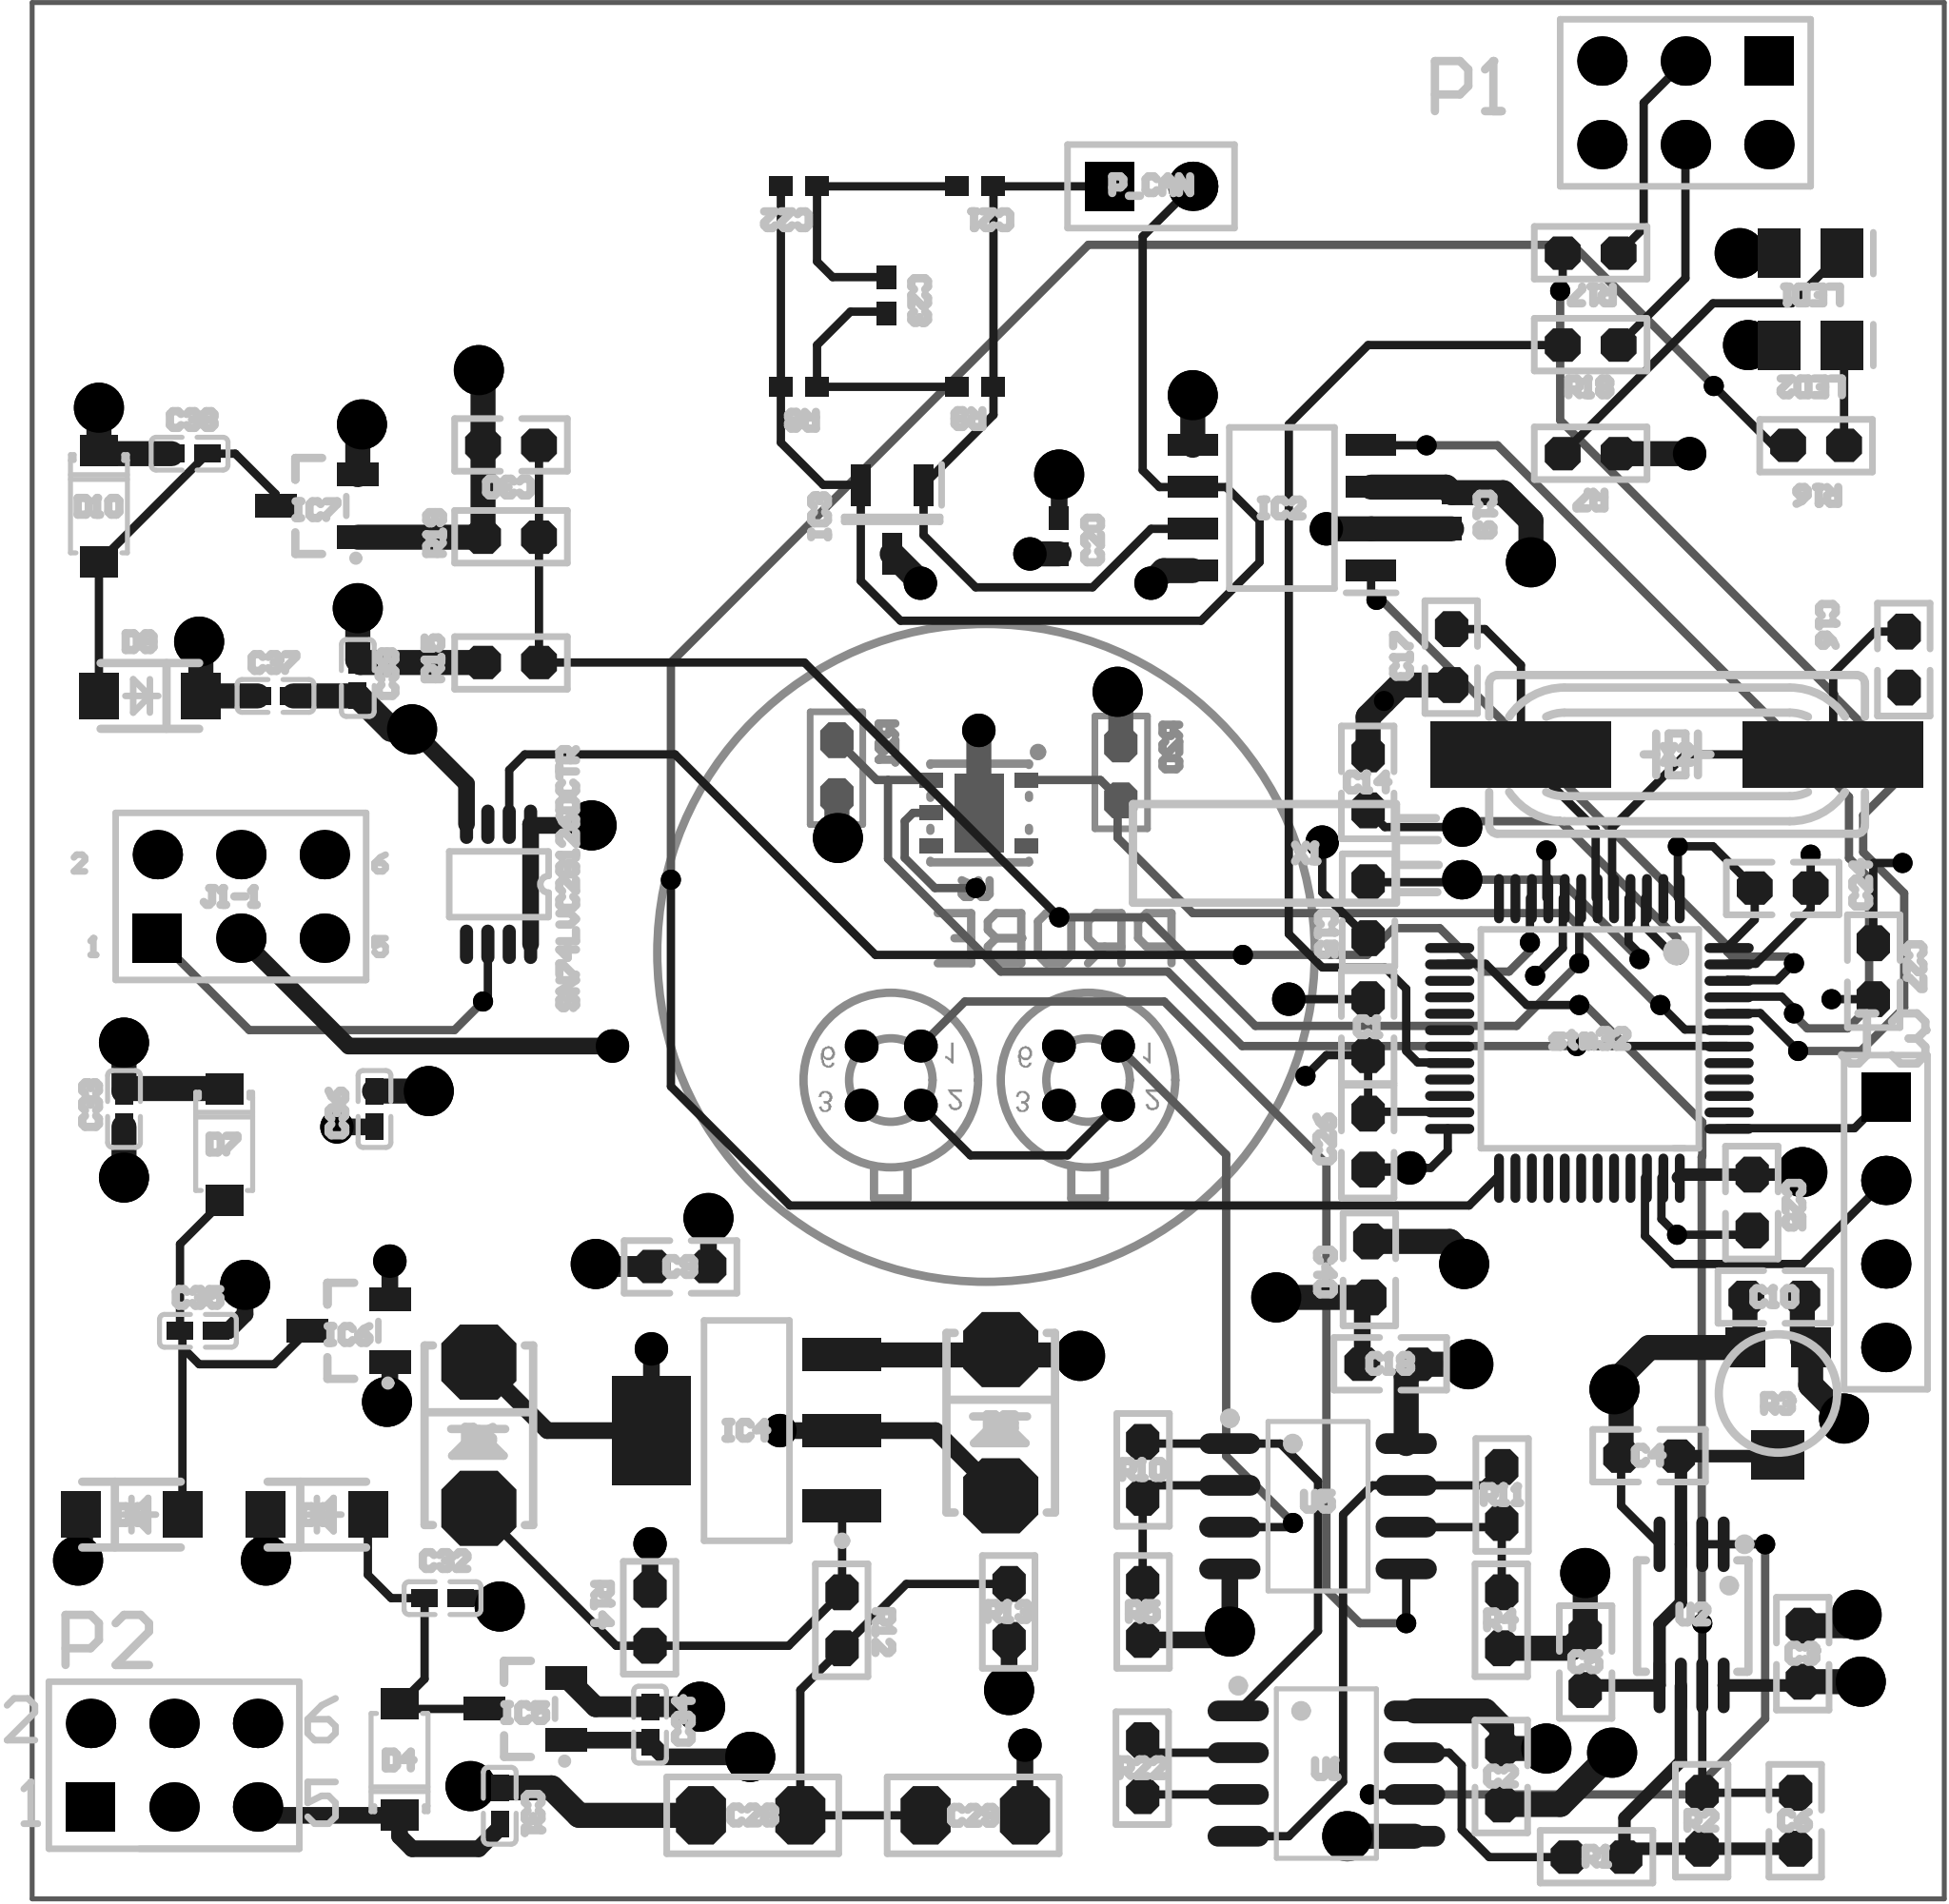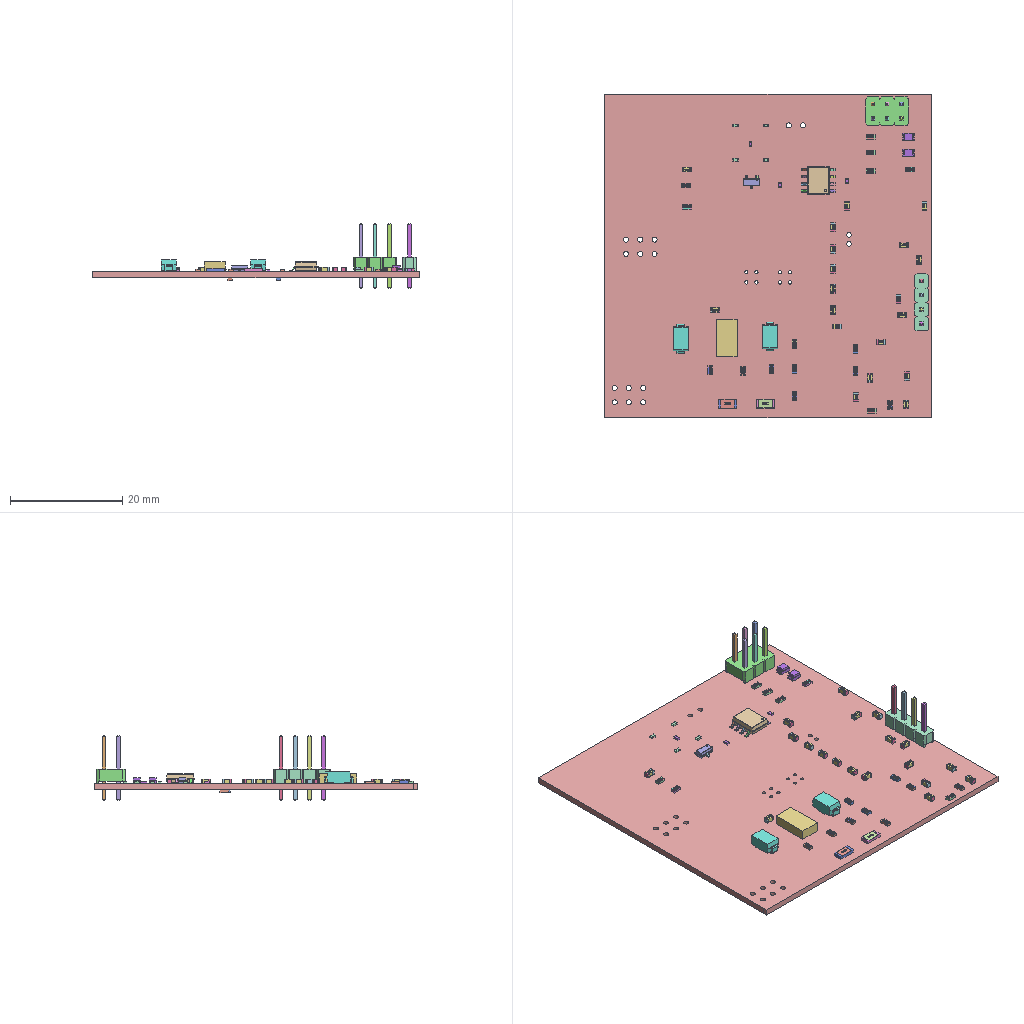Circuit board layout | Altium Designer | box 58.2 x 57.7 x 11.5 mm
Layer stack:
# Altium Designer layer stack of  (unit mm; dielectric type: 0 none, 1 core, 2 prepreg, 3 surface material)
index,name,kind,layer,copper_thickness_mm,dielectric_type,dielectric_thickness_mm,dielectric_material,dielectric_constant
0,Top Paste,other,,,,,,
1,Top Overlay,other,,,,,,
2,Top Solder,dielectric,,,3,0.0102,Solder Resist,3.5
3,Top Layer,copper,Top Layer,0.0356,,,,
4,Dielectric1,dielectric,,,1,0.254,FR-4,4.2
5,Dielectric4,dielectric,,,0,0.32,FR-4,4.8
6,GND,copper,GND,0.035,,,,
7,Dielectric 2,dielectric,,,2,0.127,,4.2
8,VCC,copper,VCC,0.035,,,,
9,Dielectric 2,dielectric,,,2,0.127,,4.2
10,Bottom Layer,copper,Bottom Layer,0.0356,,,,
11,Bottom Solder,dielectric,,,3,0.0102,Solder Resist,3.5
12,Bottom Overlay,other,,,,,,
13,Bottom Paste,other,,,,,,
# drill layer pairs: low layer,high layer
drill_pair,Top Layer,Bottom Layer
Part placement:
Designator,Comment,Layer,Footprint,Center-X(mm),Center-Y(mm),Rotation
PROBE,Header 4X2,BottomLayer,PROBE,29.12,25.03,0
P2,Header 3X2,TopLayer,HDR2X3,4.318,4.064,360
P1,Header 3*2,TopLayer,HDR3X2,50.292,54.61,180
J3,SW debug pin,TopLayer,HDR4X1_A,56.388,20.574,270
R22,953R,TopLayer,C_R0603,33.782,3.975,90
C1,Cap,TopLayer,C_C0603_M,40.64,26.505,90
C2,Cap,TopLayer,C_C0603_M,44.704,3.721,90
C3,Cap,TopLayer,C_C0603_M,53.848,7.455,270
C4,Cap,TopLayer,C_C0603_M,49.187,13.462,360
C5,0.1uF,TopLayer,C_C0603_M,47.244,7.201,270
C6,Cap,TopLayer,C_C0603_M,53.645,2.375,90
C9,Cap,TopLayer,C_C0603_M,19.723,19.228,180
C10,Cap,TopLayer,C_C0603_M,52.997,18.288,360
C14,10pF,TopLayer,C_C0603_M,40.64,33.947,90
C15,10pF,TopLayer,C_C0603_M,40.64,30.061,270
C16,22pF,TopLayer,C_C0603_M,56.947,37.681,90
C17,22pF,TopLayer,C_C0603_M,43.18,37.757,90
C18,Cap,TopLayer,C_C0603_M,41.313,16.256,360
C19,100nF,TopLayer,CAPC1005X37N,43.18,42.206,90
C20,100nF,TopLayer,CAPC1005X37N,31.242,41.444,90
C21,100pF,TopLayer,CAPC1005X37N,28.694,52.07,360
C22,100pF,TopLayer,CAPC1005X37N,23.326,52.07,360
C23,4.7nF,TopLayer,CAPC1005X37N,25.981,48.76,90
C24,100nF,TopLayer,C_C0603_M,53.251,30.734,180
C25,0.1uF,TopLayer,C_C0603_M,52.324,21.171,90
C26,100nF,TopLayer,C_C0603_M,40.64,23.025,90
C27,100nF,TopLayer,C_C0603_M,56.007,28.207,270
C28,10uF,TopLayer,C_R1206,21.857,2.54,360
C29,10uF,TopLayer,C_R1206,28.689,2.54,180
C30,1uF,TopLayer,C_C0603_M,14.567,44.196,360
C31,Cap0402,TopLayer,C0402,14.224,2.831,90
C32,Cap0402,TopLayer,C0402,12.483,9.144,180
C33,Cap0402,TopLayer,C0402,2.794,24.017,270
C34,Cap0402,TopLayer,C0402,18.796,5.297,90
C35,Cap0402,TopLayer,C0402,5.043,17.272,180
C36,Cap0402,TopLayer,C0402,10.414,24.017,270
D3,GS1004FL,TopLayer,GS1004FL,8.662,11.684,360
D4,PTVS36VS1UTR,TopLayer,PTVS36VS1UTR,11.176,4.232,90
D5,IN4007,TopLayer,C_DO-214AC,29.464,14.478,270
D6,IN4007,TopLayer,C_DO-214AC,13.589,14.097,270
D7,PTVS36VS1UTR,TopLayer,PTVS36VS1UTR,5.842,22.946,270
D8,GS1004FL,TopLayer,GS1004FL,3.022,11.684,0
IC2,TJA1051T_1J,TopLayer,SOIC-8,38.018,42.291,180
IC3,NUP2105LT1G,TopLayer,SOT-23A-3,26.162,41.944,270
IC4,LM317DCY,TopLayer,SOT223A,21.738,14.238,90
IC5,MCP1792T-5002H_CB,TopLayer,MCP1792T-220,15.006,5.776,0
IC6,MCP1792T-2.2V,TopLayer,MCP1792T-220,9.632,17.272,360
J1-1,source_select,TopLayer,HDR2X3,6.35,30.48,360
LED1,LED0,TopLayer,LED_0805_Blue,54.102,50.038,360
LED2,LED0,TopLayer,LED_0805_Blue,54.102,47.244,360
P_CAN,Header 2,TopLayer,HDR1X2,34.036,52.07,360
R1,10K,TopLayer,C_R0603,47.587,1.27,360
R2,24.9K,TopLayer,C_R0603,50.8,2.375,90
R3,100K,TopLayer,VG039N,53.102,15.139,180
R4,10K,TopLayer,C_R0603,44.704,8.471,90
R5,10K,TopLayer,C_R0603,33.782,8.725,270
R7,620,TopLayer,C_R0603,47.409,43.942,360
R8,62R,TopLayer,R0402,23.326,45.974,360
R9,62R,TopLayer,R0402,28.694,45.974,360
R10,30K,TopLayer,C_R0603,33.782,13.043,270
R11,30K,TopLayer,C_R0603,44.704,12.281,270
R12,13K,TopLayer,C_R0603,24.638,8.471,90
R13,300,TopLayer,C_R0603,29.718,8.725,90
R14,25.5k,TopLayer,C_R0603,18.796,8.547,90
R15,10K,TopLayer,C_R0603,14.567,37.592,180
R16,620,TopLayer,C_R0603,54.267,44.196,180
R17,100k,TopLayer,C_R0603,47.409,50.038,360
R18,100k,TopLayer,C_R0603,47.409,47.244,360
SN74LVC2G126DCTR,SN74LVC2G126DCTR,TopLayer,SN74LVC2G126DCTR1,14.188,30.849,180
stm32,STM32F103C8T6,TopLayer,STM32F103C8T6,47.371,26.162,180
U2,ADA4096-2ARMZ,TopLayer,ADA4096-2ARMZ,50.48,8.636,180
U5,AD8539ARZ,TopLayer,AD8422ARZ,39.116,11.938,270
X1,32.768KHz,TopLayer,直插晶振-32.768khz,43.487,31.788,360
X2,8M,TopLayer,HC-49S_L11.4-W4.8-8HZ,50.038,34.798,180
C37,Cap0402,TopLayer,C0402,7.403,36.576,180
C38,Cap0402,TopLayer,C0402,4.789,43.942,360
C39,Cap0402,TopLayer,C0402,9.906,37.121,90
D9,GS1004FL,TopLayer,GS1004FL,3.582,36.576,180
D10,PTVS36VS1UTR,TopLayer,PTVS36VS1UTR,2.032,42.332,270
IC7,MCP1792T-3.3V,TopLayer,MCP1792T-220,8.656,42.352,0
R19,0R,TopLayer,C_R0603,14.567,41.402,360
C40,Cap,TopLayer,C_C0603_M,40.691,19.139,90
U1,AD8422ARZ,TopLayer,AD8422ARZ,39.37,3.81,270
U6,HTU21D,BottomLayer,htu21d,28.798,33.02,270
R20,4.7K,BottomLayer,C_R0603,33.116,34.251,90
R21,4.7K,BottomLayer,C_R0603,24.48,34.379,270
Pad and via stacks:
# Altium Designer via and pad stacks of  (unit mm). Each distinct definition once, with the count of objects using it.
# via: kind,start_layer,end_layer,hole_mm,diameter_mm,mode(0 simple;1 top-mid-bottom;2 full stack),diameter_per_layer,count,example_net
# pad: kind,layer,hole_mm,hole_type(0 round;1 square;2 slot),plating,top_size,top_shape(1 round;2 rect;3 octagon;9 rounded rect),mid_size,bottom_size,mode,footprint,size_per_layer,count,example
pad,Top Layer,0,0,plated,0.364x1.692,1,0.364x1.692,0.364x1.692,0,ADA4096-2ARMZ,,8,U2.4
pad,Top Layer,0,0,plated,1.2x0.4,1,1.2x0.4,1.2x0.4,0,SN74LVC2G126DCTR1,,8,SN74LVC2G126DCTR.1
pad,Top Layer,0,0,plated,0.7901x0.54,2,0.7901x0.54,0.7901x0.54,0,C0402,,18,C33.2
pad,Top Layer,0,0,plated,0.7x1.25,2,0.7x1.25,0.7x1.25,0,MCP1792T-220,,9,IC5.2
pad,Top Layer,0,0,plated,1.525x0.65,2,1.525x0.65,1.525x0.65,0,SOIC-8,,8,IC2.3
pad,Top Layer,0,0,plated,1.016x1.092,3,1.016x1.092,1.016x1.092,0,C_C0603_M,,38,C9.1
pad,Top Layer,0,0,unplated,0.7x0.6,2,0.7x0.6,0.7x0.6,0,CAPC1005X37N,,10,C20.2
pad,Top Layer,0,0,plated,0.63x1.865,1,0.63x1.865,0.63x1.865,0,AD8422ARZ,,16,U5.8
pad,Top Layer,0,0,plated,2.286x2.286,3,2.286x2.286,2.286x2.286,0,C_DO-214AC,,4,D5.2
pad,Top Layer,0,0,plated,1x2.4,2,1x2.4,1x2.4,0,SOT223A,,3,IC4.3
pad,Top Layer,0,0,plated,1.2x1.4,2,1.2x1.4,1.2x1.4,0,GS1004FL,,6,D3.1
pad,Top Layer,0,0,plated,0.95x1.15,2,0.95x1.15,0.95x1.15,0,PTVS36VS1UTR,,6,D7.1
pad,Top Layer,0,0,plated,1.016x1.092,3,1.016x1.092,1.016x1.092,0,C_R0603,,32,R15.2
pad,Top Layer,0,0,unplated,1.25x0.6,2,1.25x0.6,1.25x0.6,0,SOT-23A-3,,3,IC3.3
pad,Top Layer,0,0,plated,1.2x1.2,2,1.2x1.2,1.2x1.2,0,VG039N,,2,R3.1
pad,Top Layer,0,0,plated,1.5x1.3,2,1.5x1.3,1.5x1.3,0,LED_0805_Blue,,4,LED2.1
pad,Top Layer,0,0,plated,0.3x1.5,1,0.3x1.5,0.3x1.5,0,STM32F103C8T6,,48,stm32.24
pad,Top Layer,0,0,plated,1.778x1.524,3,1.778x1.524,1.778x1.524,0,C_R1206,,4,C28.1
pad,Top Layer,0,0,plated,5.5x2,2,5.5x2,5.5x2,0,HC-49S_L11.4-W4.8-8HZ,,2,X2.1
pad,Top Layer,0,0,plated,3.3x2.4,2,3.3x2.4,3.3x2.4,0,SOT223A,,1,IC4.4
pad,Top Layer,0,0,plated,1.6x1.5,2,1.6x1.5,1.6x1.5,0,VG039N,,1,R3.2
pad,Top Layer,0,0,unplated,0.7x0.6,2,0.7x0.6,0.7x0.6,0,R0402,,4,R9.1
pad,Bottom Layer,0,0,plated,0.45x0.701,2,0.45x0.701,0.45x0.701,0,htu21d,,5,U6.5
pad,Bottom Layer,0,0,plated,1.016x1.092,3,1.016x1.092,1.016x1.092,0,C_R0603,,4,R21.2
pad,Bottom Layer,0,0,plated,2.4x1.5,2,2.4x1.5,2.4x1.5,0,htu21d,,1,U6.7
pad,Multi-Layer,0.6,0,plated,1x1,1,1x1,1x1,0,PROBE,,8,PROBE.6
pad,Multi-Layer,0.9,0,plated,1.5x1.5,2,1.5x1.5,1.5x1.5,0,HDR4X1_A,,1,J3.1
pad,Multi-Layer,0.9,0,plated,1.5x1.5,1,1.5x1.5,1.5x1.5,0,HDR4X1_A,,3,J3.2
pad,Multi-Layer,0.8,0,plated,1.2x1.2,1,1.2x1.2,1.2x1.2,0,\u00D6\u00B1\u00B2\u00E5\u00BE\u00A7\u00D5\u00F1-32.768khz,,2,X1.2
pad,Multi-Layer,0.9,0,plated,1.5x1.5,2,1.5x1.5,1.5x1.5,0,HDR2X3,,2,J1-1.1
pad,Multi-Layer,0.9,0,plated,1.5x1.5,1,1.5x1.5,1.5x1.5,0,HDR2X3,,10,J1-1.2
pad,Multi-Layer,0.9,0,plated,1.5x1.5,2,1.5x1.5,1.5x1.5,0,HDR1X2,,1,P_CAN.1
pad,Multi-Layer,0.9,0,plated,1.5x1.5,1,1.5x1.5,1.5x1.5,0,HDR1X2,,1,P_CAN.2
pad,Multi-Layer,0.9,0,plated,1.5x1.5,1,1.5x1.5,1.5x1.5,0,HDR3X2,,5,P1.6
pad,Multi-Layer,0.9,0,plated,1.5x1.5,2,1.5x1.5,1.5x1.5,0,HDR3X2,,1,P1.1
via,Top Layer,Bottom Layer,0.762,1.524,0,,42,5V
via,Top Layer,Bottom Layer,0.508,1.016,0,,16,Vin
via,Top Layer,Bottom Layer,0.3048,0.6096,0,,34,PA4
Design rules, without the lines most boards share:
# Altium Designer design rules of  (exported by Altium Designer, unit mm)
# columns: name | kind | enabled | priority | scope1 | scope2 | descriptor | typed fields (field=value)
Clearance | 0 | enabled | 1 | All | All | Clearance Constraint (Gap=0mil) (All),(All) | gap=0
PlaneConnect | 6 | enabled | 1 | All | All | Power Plane Connect Rule(Relief Connect )(Expansion=20mil) (Conductor Width=10mil) (Air Gap=10mil) (Entries=4) (All) | relief_conductor_width=0.254 relief_entries=4 relief_expansion=0.508
PolygonConnect | 20 | enabled | 1 | All | All | Polygon Connect Rule(Relief Connect )(Conductor Width=10mil) (Relief Angle=90 Angle) (Entries=4) (Air Gap Width=10mil) (All),(All) | connect_style(0=relief,1=direct,2=none)=0 relief_conductor_width=0.254 relief_entries=4
Width | 2 | enabled | 1 | All | All | Width Constraint (Min=10mil) (Max=30mil) (Preferred=10mil) (All) |
RoutingVias | 11 | enabled | 1 | All | All | Routing Via (MinHoleWidth=12mil) (MaxHoleWidth=12mil) (PreferredHoleWidth=28mil) (MinWidth=24mil) (MaxWidth=24mil) (PreferedWidth=50mil) (All) | via_min_hole=0.3048 via_max_hole=0.3048 via_preferred_diameter=1.27 via_preferred_hole=0.7112
SolderMaskExpansion | 13 | enabled | 1 | All | All | Solder Mask Expansion (Expansion =4mil) (All) | expansion=0.1016
FabricationTestpoint | 43 | enabled | 1 | (IsPad And (OnTopLayer Or OnBottomLayer)) | All | Fabrication Testpoint Style (Under Component=Yes) ((IsPad And (OnTopLayer Or OnBottomLayer))) |
ComponentClearance | 24 | enabled | 1 | All | All | Component Clearance Constraint ( Horizontal Gap = 0mil, Vertical Gap = 10mil ) (All),(All)  | gap=0
DiffPairsRouting | 51 | enabled | 1 | All | All | Differential Pairs Uncoupled Length using the Gap Constraints (Min=10mil) (Max=10mil) (Prefered=10mil)  and Width Constraints (Min=15mil) (Max=15mil) (Prefered=15mil) (All) |
HoleToHoleClearance | 52 | enabled | 1 | All | All | Hole To Hole Clearance (Gap=0mil) (All),(All) | gap=0
MinimumSolderMaskSliver | 53 | enabled | 1 | All | All | Minimum Solder Mask Sliver (Gap=0mil) (All),(All) |
SilkToSolderMaskClearance | 54 | enabled | 1 | IsPad | All | Silk To Solder Mask (Clearance=0mil) (IsPad),(All) |
SilkToSilkClearance | 55 | enabled | 1 | All | All | Silk to Silk (Clearance=0mil) (All),(All) |
Classes set for this board:
# Altium Designer classes of  (member kind: 0 net, 1 component, 2 from-to, 3 pad, 4 layer, 5 differential pair, 6 design channel, 7 polygon, 8 structure, 9 xSignal)
# columns: class name | member kind | superclass | members
Copy of JH1 | 1 | no | C1; C2; C3; C4; C5; C6; C9; C10; C14; C15; C16; C17; C18; C19; C20; C21; C22; C23; C24; C25; C26; C27; C28; C29; C30; C31; C32; C33; C34; C35; C36; D3; D4; D5; D6; D7; D8; IC2; IC3; IC4; IC5; IC6; J1-1; LED1; LED2; P_CAN; R1; R2; R3; R4; R5; R7; R8; R9; R10; R11; R12; R13; R14; R15; R16; R17; R18; SN74LVC2G126DCTR; stm32; U2; U5; X1; X2; C37; C38; C39; D9; D10; R19; IC7; U6; C40; R20; R21; R22; U1; J3; P1; P2; PROBE;